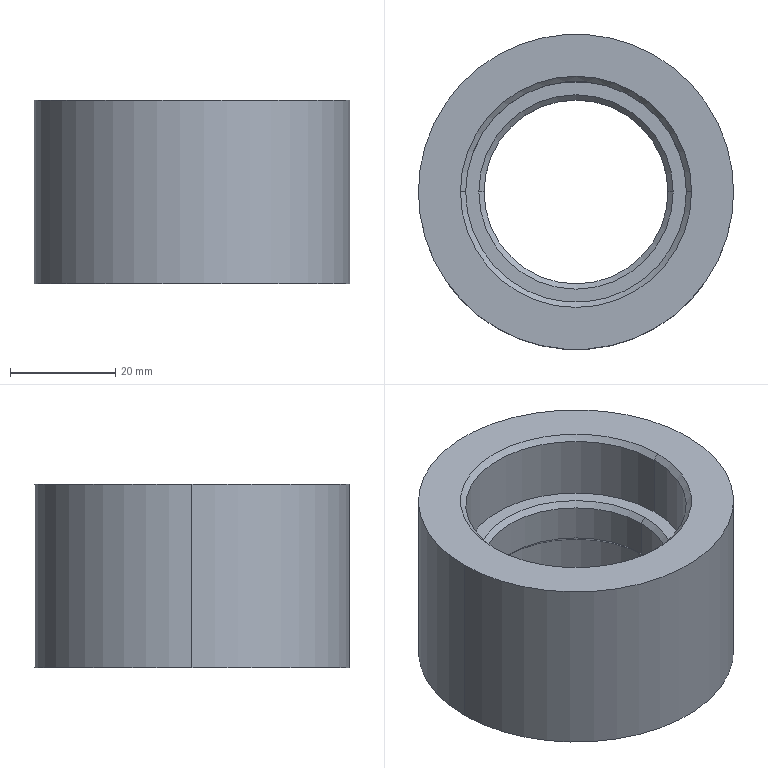Part | SolidWorks | features Chamfer 1, Extrusion 1, ICE 1, MirrorPattern 1 | 1 solid | 20 faces | box 60 x 60 x 35 mm | volume 54034 mm3 | cone 8 | cylinder 8 | plane 4 | commonest cylinder face diameters 42 x4 35 x2 60 x2
STEP:
#1=CARTESIAN_POINT('',(17.5,0.,-3.5));
#2=VERTEX_POINT('',#1);
#3=CARTESIAN_POINT('',(-17.5,0.,-3.5));
#4=VERTEX_POINT('',#3);
#5=CARTESIAN_POINT('',(0.,0.,-3.5));
#6=DIRECTION('',(0.,0.,-1.));
#7=DIRECTION('',(-1.,0.,0.));
#8=AXIS2_PLACEMENT_3D('',#5,#6,#7);
#9=CIRCLE('',#8,17.5);
#10=EDGE_CURVE('',#2,#4,#9,.T.);
#11=ORIENTED_EDGE('',*,*,#10,.F.);
#12=CARTESIAN_POINT('',(18.5,0.,-4.5));
#13=VERTEX_POINT('',#12);
#14=CARTESIAN_POINT('',(17.5,0.,-3.5));
#15=DIRECTION('',(0.7071,0.,-0.7071));
#16=VECTOR('',#15,1000.);
#17=LINE('',#14,#16);
#18=EDGE_CURVE('',#2,#13,#17,.T.);
#19=ORIENTED_EDGE('',*,*,#18,.T.);
#20=CARTESIAN_POINT('',(-18.5,0.,-4.5));
#21=VERTEX_POINT('',#20);
#22=CARTESIAN_POINT('',(0.,0.,-4.5));
#23=DIRECTION('',(0.,0.,1.));
#24=DIRECTION('',(-1.,0.,0.));
#25=AXIS2_PLACEMENT_3D('',#22,#23,#24);
#26=CIRCLE('',#25,18.5);
#27=EDGE_CURVE('',#21,#13,#26,.T.);
#28=ORIENTED_EDGE('',*,*,#27,.F.);
#29=CARTESIAN_POINT('',(-17.5,0.,-3.5));
#30=DIRECTION('',(-0.7071,0.,-0.7071));
#31=VECTOR('',#30,1000.);
#32=LINE('',#29,#31);
#33=EDGE_CURVE('',#4,#21,#32,.T.);
#34=ORIENTED_EDGE('',*,*,#33,.F.);
#35=EDGE_LOOP('',(#11,#19,#28,#34));
#36=FACE_OUTER_BOUND('',#35,.T.);
#37=CARTESIAN_POINT('',(0.,0.,-3.5));
#38=DIRECTION('',(0.,0.,-1.));
#39=DIRECTION('',(-1.,0.,0.));
#40=AXIS2_PLACEMENT_3D('',#37,#38,#39);
#41=CONICAL_SURFACE('',#40,17.5,0.7854);
#42=ADVANCED_FACE('',(#36),#41,.F.);
#43=CARTESIAN_POINT('',(21.,0.,-16.5));
#44=VERTEX_POINT('',#43);
#45=CARTESIAN_POINT('',(-21.,0.,-16.5));
#46=VERTEX_POINT('',#45);
#47=CARTESIAN_POINT('',(0.,0.,-16.5));
#48=DIRECTION('',(0.,0.,-1.));
#49=DIRECTION('',(1.,0.,0.));
#50=AXIS2_PLACEMENT_3D('',#47,#48,#49);
#51=CIRCLE('',#50,21.);
#52=EDGE_CURVE('',#44,#46,#51,.T.);
#53=ORIENTED_EDGE('',*,*,#52,.F.);
#54=CARTESIAN_POINT('',(22.,0.,-17.5));
#55=VERTEX_POINT('',#54);
#56=CARTESIAN_POINT('',(22.,0.,-17.5));
#57=DIRECTION('',(0.7071,0.,-0.7071));
#58=VECTOR('',#57,1000.);
#59=LINE('',#56,#58);
#60=EDGE_CURVE('',#44,#55,#59,.T.);
#61=ORIENTED_EDGE('',*,*,#60,.T.);
#62=CARTESIAN_POINT('',(-22.,0.,-17.5));
#63=VERTEX_POINT('',#62);
#64=CARTESIAN_POINT('',(0.,0.,-17.5));
#65=DIRECTION('',(0.,0.,1.));
#66=DIRECTION('',(1.,0.,0.));
#67=AXIS2_PLACEMENT_3D('',#64,#65,#66);
#68=CIRCLE('',#67,22.);
#69=EDGE_CURVE('',#63,#55,#68,.T.);
#70=ORIENTED_EDGE('',*,*,#69,.F.);
#71=CARTESIAN_POINT('',(-22.,0.,-17.5));
#72=DIRECTION('',(-0.7071,0.,-0.7071));
#73=VECTOR('',#72,1000.);
#74=LINE('',#71,#73);
#75=EDGE_CURVE('',#46,#63,#74,.T.);
#76=ORIENTED_EDGE('',*,*,#75,.F.);
#77=EDGE_LOOP('',(#53,#61,#70,#76));
#78=FACE_OUTER_BOUND('',#77,.T.);
#79=CARTESIAN_POINT('',(0.,0.,-17.5));
#80=DIRECTION('',(0.,0.,-1.));
#81=DIRECTION('',(-1.,0.,0.));
#82=AXIS2_PLACEMENT_3D('',#79,#80,#81);
#83=CONICAL_SURFACE('',#82,22.,0.7854);
#84=ADVANCED_FACE('',(#78),#83,.F.);
#85=CARTESIAN_POINT('',(-21.,0.,16.5));
#86=VERTEX_POINT('',#85);
#87=CARTESIAN_POINT('',(21.,0.,16.5));
#88=VERTEX_POINT('',#87);
#89=CARTESIAN_POINT('',(0.,0.,16.5));
#90=DIRECTION('',(0.,0.,1.));
#91=DIRECTION('',(1.,0.,0.));
#92=AXIS2_PLACEMENT_3D('',#89,#90,#91);
#93=CIRCLE('',#92,21.);
#94=EDGE_CURVE('',#86,#88,#93,.T.);
#95=ORIENTED_EDGE('',*,*,#94,.F.);
#96=CARTESIAN_POINT('',(-22.,0.,17.5));
#97=VERTEX_POINT('',#96);
#98=CARTESIAN_POINT('',(-21.,0.,16.5));
#99=DIRECTION('',(-0.7071,0.,0.7071));
#100=VECTOR('',#99,1000.);
#101=LINE('',#98,#100);
#102=EDGE_CURVE('',#86,#97,#101,.T.);
#103=ORIENTED_EDGE('',*,*,#102,.T.);
#104=CARTESIAN_POINT('',(22.,0.,17.5));
#105=VERTEX_POINT('',#104);
#106=CARTESIAN_POINT('',(0.,0.,17.5));
#107=DIRECTION('',(0.,0.,-1.));
#108=DIRECTION('',(1.,0.,0.));
#109=AXIS2_PLACEMENT_3D('',#106,#107,#108);
#110=CIRCLE('',#109,22.);
#111=EDGE_CURVE('',#105,#97,#110,.T.);
#112=ORIENTED_EDGE('',*,*,#111,.F.);
#113=CARTESIAN_POINT('',(21.,0.,16.5));
#114=DIRECTION('',(0.7071,0.,0.7071));
#115=VECTOR('',#114,1000.);
#116=LINE('',#113,#115);
#117=EDGE_CURVE('',#88,#105,#116,.T.);
#118=ORIENTED_EDGE('',*,*,#117,.F.);
#119=EDGE_LOOP('',(#95,#103,#112,#118));
#120=FACE_OUTER_BOUND('',#119,.T.);
#121=CARTESIAN_POINT('',(0.,0.,16.5));
#122=DIRECTION('',(0.,0.,1.));
#123=DIRECTION('',(1.,0.,0.));
#124=AXIS2_PLACEMENT_3D('',#121,#122,#123);
#125=CONICAL_SURFACE('',#124,21.,0.7854);
#126=ADVANCED_FACE('',(#120),#125,.F.);
#127=CARTESIAN_POINT('',(-17.5,0.,3.5));
#128=VERTEX_POINT('',#127);
#129=CARTESIAN_POINT('',(17.5,0.,3.5));
#130=VERTEX_POINT('',#129);
#131=CARTESIAN_POINT('',(0.,0.,3.5));
#132=DIRECTION('',(0.,0.,1.));
#133=DIRECTION('',(1.,0.,0.));
#134=AXIS2_PLACEMENT_3D('',#131,#132,#133);
#135=CIRCLE('',#134,17.5);
#136=EDGE_CURVE('',#128,#130,#135,.T.);
#137=ORIENTED_EDGE('',*,*,#136,.F.);
#138=CARTESIAN_POINT('',(-18.5,0.,4.5));
#139=VERTEX_POINT('',#138);
#140=CARTESIAN_POINT('',(-17.5,0.,3.5));
#141=DIRECTION('',(-0.7071,0.,0.7071));
#142=VECTOR('',#141,1000.);
#143=LINE('',#140,#142);
#144=EDGE_CURVE('',#128,#139,#143,.T.);
#145=ORIENTED_EDGE('',*,*,#144,.T.);
#146=CARTESIAN_POINT('',(18.5,0.,4.5));
#147=VERTEX_POINT('',#146);
#148=CARTESIAN_POINT('',(0.,0.,4.5));
#149=DIRECTION('',(0.,0.,-1.));
#150=DIRECTION('',(1.,0.,0.));
#151=AXIS2_PLACEMENT_3D('',#148,#149,#150);
#152=CIRCLE('',#151,18.5);
#153=EDGE_CURVE('',#147,#139,#152,.T.);
#154=ORIENTED_EDGE('',*,*,#153,.F.);
#155=CARTESIAN_POINT('',(17.5,0.,3.5));
#156=DIRECTION('',(0.7071,0.,0.7071));
#157=VECTOR('',#156,1000.);
#158=LINE('',#155,#157);
#159=EDGE_CURVE('',#130,#147,#158,.T.);
#160=ORIENTED_EDGE('',*,*,#159,.F.);
#161=EDGE_LOOP('',(#137,#145,#154,#160));
#162=FACE_OUTER_BOUND('',#161,.T.);
#163=CARTESIAN_POINT('',(0.,0.,3.5));
#164=DIRECTION('',(0.,0.,1.));
#165=DIRECTION('',(1.,0.,0.));
#166=AXIS2_PLACEMENT_3D('',#163,#164,#165);
#167=CONICAL_SURFACE('',#166,17.5,0.7854);
#168=ADVANCED_FACE('',(#162),#167,.F.);
#169=CARTESIAN_POINT('',(-21.,0.,-4.5));
#170=VERTEX_POINT('',#169);
#171=CARTESIAN_POINT('',(21.,0.,-4.5));
#172=VERTEX_POINT('',#171);
#173=CARTESIAN_POINT('',(0.,0.,-4.5));
#174=DIRECTION('',(0.,0.,1.));
#175=DIRECTION('',(1.,0.,0.));
#176=AXIS2_PLACEMENT_3D('',#173,#174,#175);
#177=CIRCLE('',#176,21.);
#178=EDGE_CURVE('',#170,#172,#177,.T.);
#179=ORIENTED_EDGE('',*,*,#178,.T.);
#180=CARTESIAN_POINT('',(21.,0.,-4.5));
#181=DIRECTION('',(0.,0.,-1.));
#182=VECTOR('',#181,1000.);
#183=LINE('',#180,#182);
#184=EDGE_CURVE('',#172,#44,#183,.T.);
#185=ORIENTED_EDGE('',*,*,#184,.T.);
#186=ORIENTED_EDGE('',*,*,#52,.T.);
#187=CARTESIAN_POINT('',(-21.,0.,-4.5));
#188=DIRECTION('',(0.,0.,-1.));
#189=VECTOR('',#188,1000.);
#190=LINE('',#187,#189);
#191=EDGE_CURVE('',#170,#46,#190,.T.);
#192=ORIENTED_EDGE('',*,*,#191,.F.);
#193=EDGE_LOOP('',(#179,#185,#186,#192));
#194=FACE_OUTER_BOUND('',#193,.T.);
#195=CARTESIAN_POINT('',(0.,0.,-4.5));
#196=DIRECTION('',(0.,0.,-1.));
#197=DIRECTION('',(-1.,0.,0.));
#198=AXIS2_PLACEMENT_3D('',#195,#196,#197);
#199=CYLINDRICAL_SURFACE('',#198,21.);
#200=ADVANCED_FACE('',(#194),#199,.F.);
#201=CARTESIAN_POINT('',(-21.,0.,4.5));
#202=VERTEX_POINT('',#201);
#203=CARTESIAN_POINT('',(21.,0.,4.5));
#204=VERTEX_POINT('',#203);
#205=CARTESIAN_POINT('',(0.,0.,4.5));
#206=DIRECTION('',(0.,0.,1.));
#207=DIRECTION('',(1.,0.,0.));
#208=AXIS2_PLACEMENT_3D('',#205,#206,#207);
#209=CIRCLE('',#208,21.);
#210=EDGE_CURVE('',#202,#204,#209,.T.);
#211=ORIENTED_EDGE('',*,*,#210,.F.);
#212=CARTESIAN_POINT('',(-21.,0.,4.5));
#213=DIRECTION('',(0.,0.,1.));
#214=VECTOR('',#213,1000.);
#215=LINE('',#212,#214);
#216=EDGE_CURVE('',#202,#86,#215,.T.);
#217=ORIENTED_EDGE('',*,*,#216,.T.);
#218=ORIENTED_EDGE('',*,*,#94,.T.);
#219=CARTESIAN_POINT('',(21.,0.,4.5));
#220=DIRECTION('',(0.,0.,1.));
#221=VECTOR('',#220,1000.);
#222=LINE('',#219,#221);
#223=EDGE_CURVE('',#204,#88,#222,.T.);
#224=ORIENTED_EDGE('',*,*,#223,.F.);
#225=EDGE_LOOP('',(#211,#217,#218,#224));
#226=FACE_OUTER_BOUND('',#225,.T.);
#227=CARTESIAN_POINT('',(0.,0.,4.5));
#228=DIRECTION('',(0.,0.,1.));
#229=DIRECTION('',(1.,0.,0.));
#230=AXIS2_PLACEMENT_3D('',#227,#228,#229);
#231=CYLINDRICAL_SURFACE('',#230,21.);
#232=ADVANCED_FACE('',(#226),#231,.F.);
#233=CARTESIAN_POINT('',(30.,0.,17.5));
#234=VERTEX_POINT('',#233);
#235=CARTESIAN_POINT('',(-30.,0.,17.5));
#236=VERTEX_POINT('',#235);
#237=CARTESIAN_POINT('',(0.,0.,17.5));
#238=DIRECTION('',(0.,0.,1.));
#239=DIRECTION('',(1.,0.,0.));
#240=AXIS2_PLACEMENT_3D('',#237,#238,#239);
#241=CIRCLE('',#240,30.);
#242=EDGE_CURVE('',#234,#236,#241,.T.);
#243=ORIENTED_EDGE('',*,*,#242,.F.);
#244=CARTESIAN_POINT('',(30.,0.,-17.5));
#245=VERTEX_POINT('',#244);
#246=CARTESIAN_POINT('',(30.,0.,17.5));
#247=DIRECTION('',(0.,0.,-1.));
#248=VECTOR('',#247,1000.);
#249=LINE('',#246,#248);
#250=EDGE_CURVE('',#234,#245,#249,.T.);
#251=ORIENTED_EDGE('',*,*,#250,.T.);
#252=CARTESIAN_POINT('',(-30.,0.,-17.5));
#253=VERTEX_POINT('',#252);
#254=CARTESIAN_POINT('',(0.,0.,-17.5));
#255=DIRECTION('',(0.,0.,1.));
#256=DIRECTION('',(1.,0.,0.));
#257=AXIS2_PLACEMENT_3D('',#254,#255,#256);
#258=CIRCLE('',#257,30.);
#259=EDGE_CURVE('',#245,#253,#258,.T.);
#260=ORIENTED_EDGE('',*,*,#259,.T.);
#261=CARTESIAN_POINT('',(-30.,0.,17.5));
#262=DIRECTION('',(0.,0.,-1.));
#263=VECTOR('',#262,1000.);
#264=LINE('',#261,#263);
#265=EDGE_CURVE('',#236,#253,#264,.T.);
#266=ORIENTED_EDGE('',*,*,#265,.F.);
#267=EDGE_LOOP('',(#243,#251,#260,#266));
#268=FACE_OUTER_BOUND('',#267,.T.);
#269=CARTESIAN_POINT('',(0.,0.,17.5));
#270=DIRECTION('',(0.,0.,-1.));
#271=DIRECTION('',(-1.,0.,0.));
#272=AXIS2_PLACEMENT_3D('',#269,#270,#271);
#273=CYLINDRICAL_SURFACE('',#272,30.);
#274=ADVANCED_FACE('',(#268),#273,.T.);
#275=ORIENTED_EDGE('',*,*,#136,.T.);
#276=CARTESIAN_POINT('',(17.5,0.,17.5));
#277=DIRECTION('',(0.,0.,-1.));
#278=VECTOR('',#277,1000.);
#279=LINE('',#276,#278);
#280=EDGE_CURVE('',#130,#2,#279,.T.);
#281=ORIENTED_EDGE('',*,*,#280,.T.);
#282=ORIENTED_EDGE('',*,*,#10,.T.);
#283=CARTESIAN_POINT('',(-17.5,0.,17.5));
#284=DIRECTION('',(0.,0.,-1.));
#285=VECTOR('',#284,1000.);
#286=LINE('',#283,#285);
#287=EDGE_CURVE('',#128,#4,#286,.T.);
#288=ORIENTED_EDGE('',*,*,#287,.F.);
#289=EDGE_LOOP('',(#275,#281,#282,#288));
#290=FACE_OUTER_BOUND('',#289,.T.);
#291=CARTESIAN_POINT('',(0.,0.,17.5));
#292=DIRECTION('',(0.,0.,-1.));
#293=DIRECTION('',(-1.,0.,0.));
#294=AXIS2_PLACEMENT_3D('',#291,#292,#293);
#295=CYLINDRICAL_SURFACE('',#294,17.5);
#296=ADVANCED_FACE('',(#290),#295,.F.);
#297=ORIENTED_EDGE('',*,*,#280,.F.);
#298=CARTESIAN_POINT('',(0.,0.,3.5));
#299=DIRECTION('',(0.,0.,1.));
#300=DIRECTION('',(1.,0.,0.));
#301=AXIS2_PLACEMENT_3D('',#298,#299,#300);
#302=CIRCLE('',#301,17.5);
#303=EDGE_CURVE('',#130,#128,#302,.T.);
#304=ORIENTED_EDGE('',*,*,#303,.T.);
#305=ORIENTED_EDGE('',*,*,#287,.T.);
#306=CARTESIAN_POINT('',(0.,0.,-3.5));
#307=DIRECTION('',(0.,0.,-1.));
#308=DIRECTION('',(-1.,0.,0.));
#309=AXIS2_PLACEMENT_3D('',#306,#307,#308);
#310=CIRCLE('',#309,17.5);
#311=EDGE_CURVE('',#4,#2,#310,.T.);
#312=ORIENTED_EDGE('',*,*,#311,.T.);
#313=EDGE_LOOP('',(#297,#304,#305,#312));
#314=FACE_OUTER_BOUND('',#313,.T.);
#315=CARTESIAN_POINT('',(0.,0.,17.5));
#316=DIRECTION('',(0.,0.,-1.));
#317=DIRECTION('',(-1.,0.,0.));
#318=AXIS2_PLACEMENT_3D('',#315,#316,#317);
#319=CYLINDRICAL_SURFACE('',#318,17.5);
#320=ADVANCED_FACE('',(#314),#319,.F.);
#321=ORIENTED_EDGE('',*,*,#69,.T.);
#322=CARTESIAN_POINT('',(0.,0.,-17.5));
#323=DIRECTION('',(0.,0.,1.));
#324=DIRECTION('',(1.,0.,0.));
#325=AXIS2_PLACEMENT_3D('',#322,#323,#324);
#326=CIRCLE('',#325,22.);
#327=EDGE_CURVE('',#55,#63,#326,.T.);
#328=ORIENTED_EDGE('',*,*,#327,.T.);
#329=EDGE_LOOP('',(#321,#328));
#330=FACE_BOUND('',#329,.T.);
#331=CARTESIAN_POINT('',(0.,0.,-17.5));
#332=DIRECTION('',(0.,0.,1.));
#333=DIRECTION('',(1.,0.,0.));
#334=AXIS2_PLACEMENT_3D('',#331,#332,#333);
#335=CIRCLE('',#334,30.);
#336=EDGE_CURVE('',#253,#245,#335,.T.);
#337=ORIENTED_EDGE('',*,*,#336,.F.);
#338=ORIENTED_EDGE('',*,*,#259,.F.);
#339=EDGE_LOOP('',(#337,#338));
#340=FACE_OUTER_BOUND('',#339,.T.);
#341=CARTESIAN_POINT('',(0.,0.,-17.5));
#342=DIRECTION('',(0.,0.,1.));
#343=DIRECTION('',(1.,0.,0.));
#344=AXIS2_PLACEMENT_3D('',#341,#342,#343);
#345=PLANE('',#344);
#346=ADVANCED_FACE('',(#330,#340),#345,.F.);
#347=ORIENTED_EDGE('',*,*,#111,.T.);
#348=CARTESIAN_POINT('',(0.,0.,17.5));
#349=DIRECTION('',(0.,0.,-1.));
#350=DIRECTION('',(1.,0.,0.));
#351=AXIS2_PLACEMENT_3D('',#348,#349,#350);
#352=CIRCLE('',#351,22.);
#353=EDGE_CURVE('',#97,#105,#352,.T.);
#354=ORIENTED_EDGE('',*,*,#353,.T.);
#355=EDGE_LOOP('',(#347,#354));
#356=FACE_BOUND('',#355,.T.);
#357=CARTESIAN_POINT('',(0.,0.,17.5));
#358=DIRECTION('',(0.,0.,1.));
#359=DIRECTION('',(1.,0.,0.));
#360=AXIS2_PLACEMENT_3D('',#357,#358,#359);
#361=CIRCLE('',#360,30.);
#362=EDGE_CURVE('',#236,#234,#361,.T.);
#363=ORIENTED_EDGE('',*,*,#362,.T.);
#364=ORIENTED_EDGE('',*,*,#242,.T.);
#365=EDGE_LOOP('',(#363,#364));
#366=FACE_OUTER_BOUND('',#365,.T.);
#367=CARTESIAN_POINT('',(0.,0.,17.5));
#368=DIRECTION('',(0.,0.,1.));
#369=DIRECTION('',(1.,0.,0.));
#370=AXIS2_PLACEMENT_3D('',#367,#368,#369);
#371=PLANE('',#370);
#372=ADVANCED_FACE('',(#356,#366),#371,.T.);
#373=ORIENTED_EDGE('',*,*,#250,.F.);
#374=ORIENTED_EDGE('',*,*,#362,.F.);
#375=ORIENTED_EDGE('',*,*,#265,.T.);
#376=ORIENTED_EDGE('',*,*,#336,.T.);
#377=EDGE_LOOP('',(#373,#374,#375,#376));
#378=FACE_OUTER_BOUND('',#377,.T.);
#379=CARTESIAN_POINT('',(0.,0.,17.5));
#380=DIRECTION('',(0.,0.,-1.));
#381=DIRECTION('',(-1.,0.,0.));
#382=AXIS2_PLACEMENT_3D('',#379,#380,#381);
#383=CYLINDRICAL_SURFACE('',#382,30.);
#384=ADVANCED_FACE('',(#378),#383,.T.);
#385=ORIENTED_EDGE('',*,*,#216,.F.);
#386=CARTESIAN_POINT('',(0.,0.,4.5));
#387=DIRECTION('',(0.,0.,1.));
#388=DIRECTION('',(1.,0.,0.));
#389=AXIS2_PLACEMENT_3D('',#386,#387,#388);
#390=CIRCLE('',#389,21.);
#391=EDGE_CURVE('',#204,#202,#390,.T.);
#392=ORIENTED_EDGE('',*,*,#391,.F.);
#393=ORIENTED_EDGE('',*,*,#223,.T.);
#394=CARTESIAN_POINT('',(0.,0.,16.5));
#395=DIRECTION('',(0.,0.,1.));
#396=DIRECTION('',(1.,0.,0.));
#397=AXIS2_PLACEMENT_3D('',#394,#395,#396);
#398=CIRCLE('',#397,21.);
#399=EDGE_CURVE('',#88,#86,#398,.T.);
#400=ORIENTED_EDGE('',*,*,#399,.T.);
#401=EDGE_LOOP('',(#385,#392,#393,#400));
#402=FACE_OUTER_BOUND('',#401,.T.);
#403=CARTESIAN_POINT('',(0.,0.,4.5));
#404=DIRECTION('',(0.,0.,1.));
#405=DIRECTION('',(1.,0.,0.));
#406=AXIS2_PLACEMENT_3D('',#403,#404,#405);
#407=CYLINDRICAL_SURFACE('',#406,21.);
#408=ADVANCED_FACE('',(#402),#407,.F.);
#409=ORIENTED_EDGE('',*,*,#153,.T.);
#410=CARTESIAN_POINT('',(0.,0.,4.5));
#411=DIRECTION('',(0.,0.,-1.));
#412=DIRECTION('',(1.,0.,0.));
#413=AXIS2_PLACEMENT_3D('',#410,#411,#412);
#414=CIRCLE('',#413,18.5);
#415=EDGE_CURVE('',#139,#147,#414,.T.);
#416=ORIENTED_EDGE('',*,*,#415,.T.);
#417=EDGE_LOOP('',(#409,#416));
#418=FACE_BOUND('',#417,.T.);
#419=ORIENTED_EDGE('',*,*,#391,.T.);
#420=ORIENTED_EDGE('',*,*,#210,.T.);
#421=EDGE_LOOP('',(#419,#420));
#422=FACE_OUTER_BOUND('',#421,.T.);
#423=CARTESIAN_POINT('',(0.,0.,4.5));
#424=DIRECTION('',(0.,0.,1.));
#425=DIRECTION('',(1.,0.,0.));
#426=AXIS2_PLACEMENT_3D('',#423,#424,#425);
#427=PLANE('',#426);
#428=ADVANCED_FACE('',(#418,#422),#427,.T.);
#429=ORIENTED_EDGE('',*,*,#184,.F.);
#430=CARTESIAN_POINT('',(0.,0.,-4.5));
#431=DIRECTION('',(0.,0.,1.));
#432=DIRECTION('',(1.,0.,0.));
#433=AXIS2_PLACEMENT_3D('',#430,#431,#432);
#434=CIRCLE('',#433,21.);
#435=EDGE_CURVE('',#172,#170,#434,.T.);
#436=ORIENTED_EDGE('',*,*,#435,.T.);
#437=ORIENTED_EDGE('',*,*,#191,.T.);
#438=CARTESIAN_POINT('',(0.,0.,-16.5));
#439=DIRECTION('',(0.,0.,-1.));
#440=DIRECTION('',(1.,0.,0.));
#441=AXIS2_PLACEMENT_3D('',#438,#439,#440);
#442=CIRCLE('',#441,21.);
#443=EDGE_CURVE('',#46,#44,#442,.T.);
#444=ORIENTED_EDGE('',*,*,#443,.T.);
#445=EDGE_LOOP('',(#429,#436,#437,#444));
#446=FACE_OUTER_BOUND('',#445,.T.);
#447=CARTESIAN_POINT('',(0.,0.,-4.5));
#448=DIRECTION('',(0.,0.,-1.));
#449=DIRECTION('',(-1.,0.,0.));
#450=AXIS2_PLACEMENT_3D('',#447,#448,#449);
#451=CYLINDRICAL_SURFACE('',#450,21.);
#452=ADVANCED_FACE('',(#446),#451,.F.);
#453=ORIENTED_EDGE('',*,*,#27,.T.);
#454=CARTESIAN_POINT('',(0.,0.,-4.5));
#455=DIRECTION('',(0.,0.,1.));
#456=DIRECTION('',(-1.,0.,0.));
#457=AXIS2_PLACEMENT_3D('',#454,#455,#456);
#458=CIRCLE('',#457,18.5);
#459=EDGE_CURVE('',#13,#21,#458,.T.);
#460=ORIENTED_EDGE('',*,*,#459,.T.);
#461=EDGE_LOOP('',(#453,#460));
#462=FACE_BOUND('',#461,.T.);
#463=ORIENTED_EDGE('',*,*,#178,.F.);
#464=ORIENTED_EDGE('',*,*,#435,.F.);
#465=EDGE_LOOP('',(#463,#464));
#466=FACE_OUTER_BOUND('',#465,.T.);
#467=CARTESIAN_POINT('',(0.,0.,-4.5));
#468=DIRECTION('',(0.,0.,-1.));
#469=DIRECTION('',(1.,0.,0.));
#470=AXIS2_PLACEMENT_3D('',#467,#468,#469);
#471=PLANE('',#470);
#472=ADVANCED_FACE('',(#462,#466),#471,.T.);
#473=ORIENTED_EDGE('',*,*,#144,.F.);
#474=ORIENTED_EDGE('',*,*,#303,.F.);
#475=ORIENTED_EDGE('',*,*,#159,.T.);
#476=ORIENTED_EDGE('',*,*,#415,.F.);
#477=EDGE_LOOP('',(#473,#474,#475,#476));
#478=FACE_OUTER_BOUND('',#477,.T.);
#479=CARTESIAN_POINT('',(0.,0.,3.5));
#480=DIRECTION('',(0.,0.,1.));
#481=DIRECTION('',(1.,0.,0.));
#482=AXIS2_PLACEMENT_3D('',#479,#480,#481);
#483=CONICAL_SURFACE('',#482,17.5,0.7854);
#484=ADVANCED_FACE('',(#478),#483,.F.);
#485=ORIENTED_EDGE('',*,*,#102,.F.);
#486=ORIENTED_EDGE('',*,*,#399,.F.);
#487=ORIENTED_EDGE('',*,*,#117,.T.);
#488=ORIENTED_EDGE('',*,*,#353,.F.);
#489=EDGE_LOOP('',(#485,#486,#487,#488));
#490=FACE_OUTER_BOUND('',#489,.T.);
#491=CARTESIAN_POINT('',(0.,0.,16.5));
#492=DIRECTION('',(0.,0.,1.));
#493=DIRECTION('',(1.,0.,0.));
#494=AXIS2_PLACEMENT_3D('',#491,#492,#493);
#495=CONICAL_SURFACE('',#494,21.,0.7854);
#496=ADVANCED_FACE('',(#490),#495,.F.);
#497=ORIENTED_EDGE('',*,*,#60,.F.);
#498=ORIENTED_EDGE('',*,*,#443,.F.);
#499=ORIENTED_EDGE('',*,*,#75,.T.);
#500=ORIENTED_EDGE('',*,*,#327,.F.);
#501=EDGE_LOOP('',(#497,#498,#499,#500));
#502=FACE_OUTER_BOUND('',#501,.T.);
#503=CARTESIAN_POINT('',(0.,0.,-17.5));
#504=DIRECTION('',(0.,0.,-1.));
#505=DIRECTION('',(-1.,0.,0.));
#506=AXIS2_PLACEMENT_3D('',#503,#504,#505);
#507=CONICAL_SURFACE('',#506,22.,0.7854);
#508=ADVANCED_FACE('',(#502),#507,.F.);
#509=ORIENTED_EDGE('',*,*,#18,.F.);
#510=ORIENTED_EDGE('',*,*,#311,.F.);
#511=ORIENTED_EDGE('',*,*,#33,.T.);
#512=ORIENTED_EDGE('',*,*,#459,.F.);
#513=EDGE_LOOP('',(#509,#510,#511,#512));
#514=FACE_OUTER_BOUND('',#513,.T.);
#515=CARTESIAN_POINT('',(0.,0.,-3.5));
#516=DIRECTION('',(0.,0.,-1.));
#517=DIRECTION('',(-1.,0.,0.));
#518=AXIS2_PLACEMENT_3D('',#515,#516,#517);
#519=CONICAL_SURFACE('',#518,17.5,0.7854);
#520=ADVANCED_FACE('',(#514),#519,.F.);
#521=CLOSED_SHELL('',(#42,#84,#126,#168,#200,#232,#274,#296,#320,#346,#372,#384,#408,#428,#452,#472,#484,#496,#508,#520));
#522=MANIFOLD_SOLID_BREP('',#521);
#523=CARTESIAN_POINT('',(0.,0.,0.));
#524=DIRECTION('',(0.,0.,1.));
#525=DIRECTION('',(1.,0.,0.));
#526=AXIS2_PLACEMENT_3D('',#523,#524,#525);
#527=(LENGTH_UNIT()NAMED_UNIT(*)SI_UNIT(.MILLI.,.METRE.));
#528=UNCERTAINTY_MEASURE_WITH_UNIT(LENGTH_MEASURE(0.00001),#527,'','');
#529=(NAMED_UNIT(*)PLANE_ANGLE_UNIT()SI_UNIT($,.RADIAN.));
#530=(NAMED_UNIT(*)SI_UNIT($,.STERADIAN.)SOLID_ANGLE_UNIT());
#531=(GEOMETRIC_REPRESENTATION_CONTEXT(3)GLOBAL_UNCERTAINTY_ASSIGNED_CONTEXT((#528))GLOBAL_UNIT_ASSIGNED_CONTEXT((#527,#529,#530))REPRESENTATION_CONTEXT('',''));
#532=ADVANCED_BREP_SHAPE_REPRESENTATION('',(#522,#526),#531);